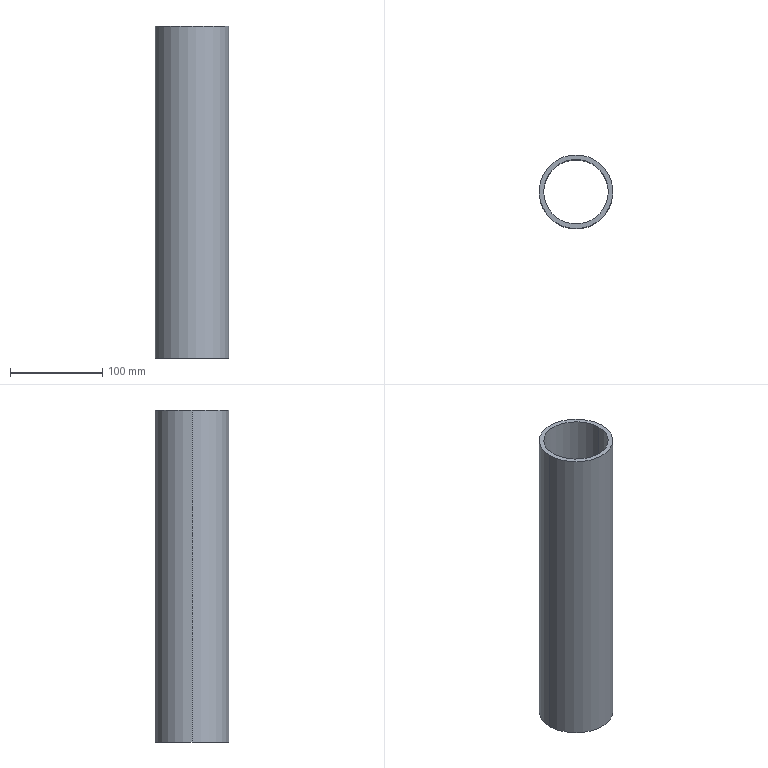Part | SolidWorks | features Extrusion 1 | 1 solid | 6 faces | box 80 x 80 x 360 mm | volume 424115 mm3 | cylinder 4 | plane 2 | commonest cylinder face diameters 70 x2 80 x2
STEP:
#1=CARTESIAN_POINT('',(-35.,0.,360.));
#2=VERTEX_POINT('',#1);
#3=CARTESIAN_POINT('',(35.,0.,360.));
#4=VERTEX_POINT('',#3);
#5=CARTESIAN_POINT('',(0.,0.,360.));
#6=DIRECTION('',(0.,0.,1.));
#7=DIRECTION('',(1.,0.,0.));
#8=AXIS2_PLACEMENT_3D('',#5,#6,#7);
#9=CIRCLE('',#8,35.);
#10=EDGE_CURVE('',#2,#4,#9,.T.);
#11=ORIENTED_EDGE('',*,*,#10,.T.);
#12=CARTESIAN_POINT('',(35.,0.,0.));
#13=VERTEX_POINT('',#12);
#14=CARTESIAN_POINT('',(35.,0.,360.));
#15=DIRECTION('',(0.,0.,-1.));
#16=VECTOR('',#15,1000.);
#17=LINE('',#14,#16);
#18=EDGE_CURVE('',#4,#13,#17,.T.);
#19=ORIENTED_EDGE('',*,*,#18,.T.);
#20=CARTESIAN_POINT('',(-35.,0.,0.));
#21=VERTEX_POINT('',#20);
#22=CARTESIAN_POINT('',(0.,0.,0.));
#23=DIRECTION('',(0.,0.,1.));
#24=DIRECTION('',(1.,0.,0.));
#25=AXIS2_PLACEMENT_3D('',#22,#23,#24);
#26=CIRCLE('',#25,35.);
#27=EDGE_CURVE('',#21,#13,#26,.T.);
#28=ORIENTED_EDGE('',*,*,#27,.F.);
#29=CARTESIAN_POINT('',(-35.,0.,360.));
#30=DIRECTION('',(0.,0.,-1.));
#31=VECTOR('',#30,1000.);
#32=LINE('',#29,#31);
#33=EDGE_CURVE('',#2,#21,#32,.T.);
#34=ORIENTED_EDGE('',*,*,#33,.F.);
#35=EDGE_LOOP('',(#11,#19,#28,#34));
#36=FACE_OUTER_BOUND('',#35,.T.);
#37=CARTESIAN_POINT('',(0.,0.,360.));
#38=DIRECTION('',(0.,0.,-1.));
#39=DIRECTION('',(-1.,0.,0.));
#40=AXIS2_PLACEMENT_3D('',#37,#38,#39);
#41=CYLINDRICAL_SURFACE('',#40,35.);
#42=ADVANCED_FACE('',(#36),#41,.F.);
#43=CARTESIAN_POINT('',(40.,0.,360.));
#44=VERTEX_POINT('',#43);
#45=CARTESIAN_POINT('',(-40.,0.,360.));
#46=VERTEX_POINT('',#45);
#47=CARTESIAN_POINT('',(0.,0.,360.));
#48=DIRECTION('',(0.,0.,1.));
#49=DIRECTION('',(1.,0.,0.));
#50=AXIS2_PLACEMENT_3D('',#47,#48,#49);
#51=CIRCLE('',#50,40.);
#52=EDGE_CURVE('',#44,#46,#51,.T.);
#53=ORIENTED_EDGE('',*,*,#52,.F.);
#54=CARTESIAN_POINT('',(40.,0.,0.));
#55=VERTEX_POINT('',#54);
#56=CARTESIAN_POINT('',(40.,0.,360.));
#57=DIRECTION('',(0.,0.,-1.));
#58=VECTOR('',#57,1000.);
#59=LINE('',#56,#58);
#60=EDGE_CURVE('',#44,#55,#59,.T.);
#61=ORIENTED_EDGE('',*,*,#60,.T.);
#62=CARTESIAN_POINT('',(-40.,0.,0.));
#63=VERTEX_POINT('',#62);
#64=CARTESIAN_POINT('',(0.,0.,0.));
#65=DIRECTION('',(0.,0.,1.));
#66=DIRECTION('',(1.,0.,0.));
#67=AXIS2_PLACEMENT_3D('',#64,#65,#66);
#68=CIRCLE('',#67,40.);
#69=EDGE_CURVE('',#55,#63,#68,.T.);
#70=ORIENTED_EDGE('',*,*,#69,.T.);
#71=CARTESIAN_POINT('',(-40.,0.,360.));
#72=DIRECTION('',(0.,0.,-1.));
#73=VECTOR('',#72,1000.);
#74=LINE('',#71,#73);
#75=EDGE_CURVE('',#46,#63,#74,.T.);
#76=ORIENTED_EDGE('',*,*,#75,.F.);
#77=EDGE_LOOP('',(#53,#61,#70,#76));
#78=FACE_OUTER_BOUND('',#77,.T.);
#79=CARTESIAN_POINT('',(0.,0.,360.));
#80=DIRECTION('',(0.,0.,-1.));
#81=DIRECTION('',(-1.,0.,0.));
#82=AXIS2_PLACEMENT_3D('',#79,#80,#81);
#83=CYLINDRICAL_SURFACE('',#82,40.);
#84=ADVANCED_FACE('',(#78),#83,.T.);
#85=CARTESIAN_POINT('',(0.,0.,360.));
#86=DIRECTION('',(0.,0.,1.));
#87=DIRECTION('',(1.,0.,0.));
#88=AXIS2_PLACEMENT_3D('',#85,#86,#87);
#89=CIRCLE('',#88,40.);
#90=EDGE_CURVE('',#46,#44,#89,.T.);
#91=ORIENTED_EDGE('',*,*,#90,.T.);
#92=ORIENTED_EDGE('',*,*,#52,.T.);
#93=EDGE_LOOP('',(#91,#92));
#94=FACE_OUTER_BOUND('',#93,.T.);
#95=ORIENTED_EDGE('',*,*,#10,.F.);
#96=CARTESIAN_POINT('',(0.,0.,360.));
#97=DIRECTION('',(0.,0.,1.));
#98=DIRECTION('',(1.,0.,0.));
#99=AXIS2_PLACEMENT_3D('',#96,#97,#98);
#100=CIRCLE('',#99,35.);
#101=EDGE_CURVE('',#4,#2,#100,.T.);
#102=ORIENTED_EDGE('',*,*,#101,.F.);
#103=EDGE_LOOP('',(#95,#102));
#104=FACE_BOUND('',#103,.T.);
#105=CARTESIAN_POINT('',(0.,0.,360.));
#106=DIRECTION('',(0.,0.,1.));
#107=DIRECTION('',(1.,0.,0.));
#108=AXIS2_PLACEMENT_3D('',#105,#106,#107);
#109=PLANE('',#108);
#110=ADVANCED_FACE('',(#94,#104),#109,.T.);
#111=CARTESIAN_POINT('',(0.,0.,0.));
#112=DIRECTION('',(0.,0.,1.));
#113=DIRECTION('',(1.,0.,0.));
#114=AXIS2_PLACEMENT_3D('',#111,#112,#113);
#115=CIRCLE('',#114,40.);
#116=EDGE_CURVE('',#63,#55,#115,.T.);
#117=ORIENTED_EDGE('',*,*,#116,.F.);
#118=ORIENTED_EDGE('',*,*,#69,.F.);
#119=EDGE_LOOP('',(#117,#118));
#120=FACE_OUTER_BOUND('',#119,.T.);
#121=ORIENTED_EDGE('',*,*,#27,.T.);
#122=CARTESIAN_POINT('',(0.,0.,0.));
#123=DIRECTION('',(0.,0.,1.));
#124=DIRECTION('',(1.,0.,0.));
#125=AXIS2_PLACEMENT_3D('',#122,#123,#124);
#126=CIRCLE('',#125,35.);
#127=EDGE_CURVE('',#13,#21,#126,.T.);
#128=ORIENTED_EDGE('',*,*,#127,.T.);
#129=EDGE_LOOP('',(#121,#128));
#130=FACE_BOUND('',#129,.T.);
#131=CARTESIAN_POINT('',(0.,0.,0.));
#132=DIRECTION('',(0.,0.,1.));
#133=DIRECTION('',(1.,0.,0.));
#134=AXIS2_PLACEMENT_3D('',#131,#132,#133);
#135=PLANE('',#134);
#136=ADVANCED_FACE('',(#120,#130),#135,.F.);
#137=ORIENTED_EDGE('',*,*,#60,.F.);
#138=ORIENTED_EDGE('',*,*,#90,.F.);
#139=ORIENTED_EDGE('',*,*,#75,.T.);
#140=ORIENTED_EDGE('',*,*,#116,.T.);
#141=EDGE_LOOP('',(#137,#138,#139,#140));
#142=FACE_OUTER_BOUND('',#141,.T.);
#143=CARTESIAN_POINT('',(0.,0.,360.));
#144=DIRECTION('',(0.,0.,-1.));
#145=DIRECTION('',(-1.,0.,0.));
#146=AXIS2_PLACEMENT_3D('',#143,#144,#145);
#147=CYLINDRICAL_SURFACE('',#146,40.);
#148=ADVANCED_FACE('',(#142),#147,.T.);
#149=ORIENTED_EDGE('',*,*,#18,.F.);
#150=ORIENTED_EDGE('',*,*,#101,.T.);
#151=ORIENTED_EDGE('',*,*,#33,.T.);
#152=ORIENTED_EDGE('',*,*,#127,.F.);
#153=EDGE_LOOP('',(#149,#150,#151,#152));
#154=FACE_OUTER_BOUND('',#153,.T.);
#155=CARTESIAN_POINT('',(0.,0.,360.));
#156=DIRECTION('',(0.,0.,-1.));
#157=DIRECTION('',(-1.,0.,0.));
#158=AXIS2_PLACEMENT_3D('',#155,#156,#157);
#159=CYLINDRICAL_SURFACE('',#158,35.);
#160=ADVANCED_FACE('',(#154),#159,.F.);
#161=CLOSED_SHELL('',(#42,#84,#110,#136,#148,#160));
#162=MANIFOLD_SOLID_BREP('',#161);
#163=CARTESIAN_POINT('',(0.,0.,0.));
#164=DIRECTION('',(0.,0.,1.));
#165=DIRECTION('',(1.,0.,0.));
#166=AXIS2_PLACEMENT_3D('',#163,#164,#165);
#167=(LENGTH_UNIT()NAMED_UNIT(*)SI_UNIT(.MILLI.,.METRE.));
#168=UNCERTAINTY_MEASURE_WITH_UNIT(LENGTH_MEASURE(0.00001),#167,'','');
#169=(NAMED_UNIT(*)PLANE_ANGLE_UNIT()SI_UNIT($,.RADIAN.));
#170=(NAMED_UNIT(*)SI_UNIT($,.STERADIAN.)SOLID_ANGLE_UNIT());
#171=(GEOMETRIC_REPRESENTATION_CONTEXT(3)GLOBAL_UNCERTAINTY_ASSIGNED_CONTEXT((#168))GLOBAL_UNIT_ASSIGNED_CONTEXT((#167,#169,#170))REPRESENTATION_CONTEXT('',''));
#172=ADVANCED_BREP_SHAPE_REPRESENTATION('',(#162,#166),#171);